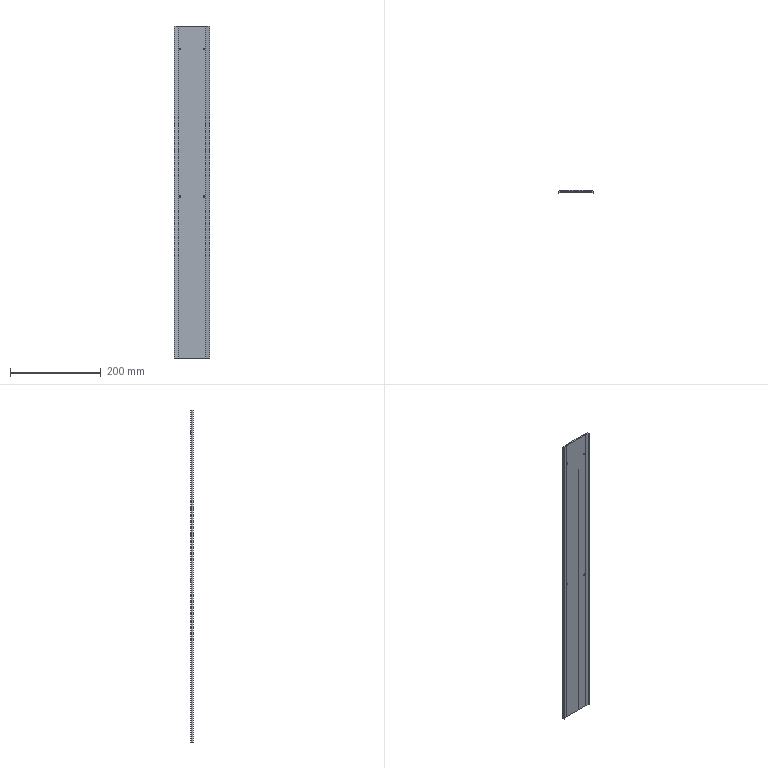Part | NX | 1 solid | 37 faces | box 79 x 6 x 732 mm | volume 149566 mm3 | plane 29 | cylinder 4 | cone 4 | commonest cylinder face diameters 3.4 x4
STEP:
#1=CARTESIAN_POINT('',(518.205,169.433,382.));
#2=VERTEX_POINT('',#1);
#3=CARTESIAN_POINT('',(518.205,165.108,382.));
#4=VERTEX_POINT('',#3);
#5=CARTESIAN_POINT('',(518.205,169.433,382.));
#6=DIRECTION('',(0.,-1.,0.));
#7=VECTOR('',#6,1.);
#8=LINE('',#5,#7);
#9=EDGE_CURVE('',#2,#4,#8,.T.);
#10=ORIENTED_EDGE('',*,*,#9,.F.);
#11=CARTESIAN_POINT('',(518.205,169.433,-350.));
#12=VERTEX_POINT('',#11);
#13=CARTESIAN_POINT('',(518.205,169.433,0.));
#14=DIRECTION('',(0.,0.,1.));
#15=VECTOR('',#14,1.);
#16=LINE('',#13,#15);
#17=EDGE_CURVE('',#12,#2,#16,.T.);
#18=ORIENTED_EDGE('',*,*,#17,.F.);
#19=CARTESIAN_POINT('',(518.205,165.108,-350.));
#20=VERTEX_POINT('',#19);
#21=CARTESIAN_POINT('',(518.205,0.,-350.));
#22=DIRECTION('',(0.,-1.,0.));
#23=VECTOR('',#22,1.);
#24=LINE('',#21,#23);
#25=EDGE_CURVE('',#12,#20,#24,.T.);
#26=ORIENTED_EDGE('',*,*,#25,.T.);
#27=CARTESIAN_POINT('',(518.205,165.108,0.));
#28=DIRECTION('',(0.,0.,1.));
#29=VECTOR('',#28,1.);
#30=LINE('',#27,#29);
#31=EDGE_CURVE('',#20,#4,#30,.T.);
#32=ORIENTED_EDGE('',*,*,#31,.T.);
#33=EDGE_LOOP('',(#10,#18,#26,#32));
#34=FACE_OUTER_BOUND('',#33,.T.);
#35=CARTESIAN_POINT('',(518.205,169.433,0.));
#36=DIRECTION('',(-1.,0.,0.));
#37=DIRECTION('',(0.,0.,-1.));
#38=AXIS2_PLACEMENT_3D('',#35,#36,#37);
#39=PLANE('',#38);
#40=ADVANCED_FACE('',(#34),#39,.T.);
#41=CARTESIAN_POINT('',(520.205,165.108,382.));
#42=VERTEX_POINT('',#41);
#43=CARTESIAN_POINT('',(518.205,165.108,382.));
#44=DIRECTION('',(1.,0.,0.));
#45=VECTOR('',#44,1.);
#46=LINE('',#43,#45);
#47=EDGE_CURVE('',#4,#42,#46,.T.);
#48=ORIENTED_EDGE('',*,*,#47,.F.);
#49=ORIENTED_EDGE('',*,*,#31,.F.);
#50=CARTESIAN_POINT('',(520.205,165.108,-350.));
#51=VERTEX_POINT('',#50);
#52=CARTESIAN_POINT('',(0.,165.108,-350.));
#53=DIRECTION('',(1.,0.,0.));
#54=VECTOR('',#53,1.);
#55=LINE('',#52,#54);
#56=EDGE_CURVE('',#20,#51,#55,.T.);
#57=ORIENTED_EDGE('',*,*,#56,.T.);
#58=CARTESIAN_POINT('',(520.205,165.108,0.));
#59=DIRECTION('',(0.,0.,1.));
#60=VECTOR('',#59,1.);
#61=LINE('',#58,#60);
#62=EDGE_CURVE('',#51,#42,#61,.T.);
#63=ORIENTED_EDGE('',*,*,#62,.T.);
#64=EDGE_LOOP('',(#48,#49,#57,#63));
#65=FACE_OUTER_BOUND('',#64,.T.);
#66=CARTESIAN_POINT('',(518.205,165.108,0.));
#67=DIRECTION('',(0.,-1.,0.));
#68=DIRECTION('',(0.,0.,1.));
#69=AXIS2_PLACEMENT_3D('',#66,#67,#68);
#70=PLANE('',#69);
#71=ADVANCED_FACE('',(#65),#70,.T.);
#72=CARTESIAN_POINT('',(520.205,167.247,382.));
#73=VERTEX_POINT('',#72);
#74=CARTESIAN_POINT('',(520.205,165.108,382.));
#75=DIRECTION('',(0.,1.,0.));
#76=VECTOR('',#75,1.);
#77=LINE('',#74,#76);
#78=EDGE_CURVE('',#42,#73,#77,.T.);
#79=ORIENTED_EDGE('',*,*,#78,.F.);
#80=ORIENTED_EDGE('',*,*,#62,.F.);
#81=CARTESIAN_POINT('',(520.205,167.247,-350.));
#82=VERTEX_POINT('',#81);
#83=CARTESIAN_POINT('',(520.205,0.,-350.));
#84=DIRECTION('',(0.,1.,0.));
#85=VECTOR('',#84,1.);
#86=LINE('',#83,#85);
#87=EDGE_CURVE('',#51,#82,#86,.T.);
#88=ORIENTED_EDGE('',*,*,#87,.T.);
#89=CARTESIAN_POINT('',(520.205,167.247,0.));
#90=DIRECTION('',(0.,0.,1.));
#91=VECTOR('',#90,1.);
#92=LINE('',#89,#91);
#93=EDGE_CURVE('',#82,#73,#92,.T.);
#94=ORIENTED_EDGE('',*,*,#93,.T.);
#95=EDGE_LOOP('',(#79,#80,#88,#94));
#96=FACE_OUTER_BOUND('',#95,.T.);
#97=CARTESIAN_POINT('',(520.205,165.108,0.));
#98=DIRECTION('',(1.,0.,0.));
#99=DIRECTION('',(0.,0.,1.));
#100=AXIS2_PLACEMENT_3D('',#97,#98,#99);
#101=PLANE('',#100);
#102=ADVANCED_FACE('',(#96),#101,.T.);
#103=CARTESIAN_POINT('',(527.924,168.608,382.));
#104=VERTEX_POINT('',#103);
#105=CARTESIAN_POINT('',(520.205,167.247,382.));
#106=DIRECTION('',(0.9848,0.1736,0.));
#107=VECTOR('',#106,1.);
#108=LINE('',#105,#107);
#109=EDGE_CURVE('',#73,#104,#108,.T.);
#110=ORIENTED_EDGE('',*,*,#109,.F.);
#111=ORIENTED_EDGE('',*,*,#93,.F.);
#112=CARTESIAN_POINT('',(527.924,168.608,-350.));
#113=VERTEX_POINT('',#112);
#114=CARTESIAN_POINT('',(-12.915,73.244,-350.));
#115=DIRECTION('',(0.9848,0.1736,0.));
#116=VECTOR('',#115,1.);
#117=LINE('',#114,#116);
#118=EDGE_CURVE('',#82,#113,#117,.T.);
#119=ORIENTED_EDGE('',*,*,#118,.T.);
#120=CARTESIAN_POINT('',(527.924,168.608,0.));
#121=DIRECTION('',(0.,0.,1.));
#122=VECTOR('',#121,1.);
#123=LINE('',#120,#122);
#124=EDGE_CURVE('',#113,#104,#123,.T.);
#125=ORIENTED_EDGE('',*,*,#124,.T.);
#126=EDGE_LOOP('',(#110,#111,#119,#125));
#127=FACE_OUTER_BOUND('',#126,.T.);
#128=CARTESIAN_POINT('',(520.205,167.247,0.));
#129=DIRECTION('',(0.1736,-0.9848,0.));
#130=DIRECTION('',(-0.9848,-0.1736,0.));
#131=AXIS2_PLACEMENT_3D('',#128,#129,#130);
#132=PLANE('',#131);
#133=ADVANCED_FACE('',(#127),#132,.T.);
#134=CARTESIAN_POINT('',(531.705,168.608,329.8));
#135=VERTEX_POINT('',#134);
#136=CARTESIAN_POINT('',(531.705,168.608,331.5));
#137=DIRECTION('',(0.,-1.,0.));
#138=DIRECTION('',(0.,0.,-1.));
#139=AXIS2_PLACEMENT_3D('',#136,#137,#138);
#140=CIRCLE('',#139,1.7);
#141=EDGE_CURVE('',#135,#135,#140,.T.);
#142=ORIENTED_EDGE('',*,*,#141,.F.);
#143=EDGE_LOOP('',(#142));
#144=FACE_BOUND('',#143,.T.);
#145=CARTESIAN_POINT('',(583.705,168.608,4.3));
#146=VERTEX_POINT('',#145);
#147=CARTESIAN_POINT('',(583.705,168.608,6.));
#148=DIRECTION('',(0.,-1.,0.));
#149=DIRECTION('',(0.,0.,-1.));
#150=AXIS2_PLACEMENT_3D('',#147,#148,#149);
#151=CIRCLE('',#150,1.7);
#152=EDGE_CURVE('',#146,#146,#151,.T.);
#153=ORIENTED_EDGE('',*,*,#152,.F.);
#154=EDGE_LOOP('',(#153));
#155=FACE_BOUND('',#154,.T.);
#156=CARTESIAN_POINT('',(583.705,168.608,329.8));
#157=VERTEX_POINT('',#156);
#158=CARTESIAN_POINT('',(583.705,168.608,331.5));
#159=DIRECTION('',(0.,-1.,0.));
#160=DIRECTION('',(0.,0.,-1.));
#161=AXIS2_PLACEMENT_3D('',#158,#159,#160);
#162=CIRCLE('',#161,1.7);
#163=EDGE_CURVE('',#157,#157,#162,.T.);
#164=ORIENTED_EDGE('',*,*,#163,.F.);
#165=EDGE_LOOP('',(#164));
#166=FACE_BOUND('',#165,.T.);
#167=CARTESIAN_POINT('',(531.705,168.608,4.3));
#168=VERTEX_POINT('',#167);
#169=CARTESIAN_POINT('',(531.705,168.608,6.));
#170=DIRECTION('',(0.,-1.,0.));
#171=DIRECTION('',(0.,0.,-1.));
#172=AXIS2_PLACEMENT_3D('',#169,#170,#171);
#173=CIRCLE('',#172,1.7);
#174=EDGE_CURVE('',#168,#168,#173,.T.);
#175=ORIENTED_EDGE('',*,*,#174,.F.);
#176=EDGE_LOOP('',(#175));
#177=FACE_BOUND('',#176,.T.);
#178=CARTESIAN_POINT('',(587.487,168.608,382.));
#179=VERTEX_POINT('',#178);
#180=CARTESIAN_POINT('',(527.924,168.608,382.));
#181=DIRECTION('',(1.,0.,0.));
#182=VECTOR('',#181,1.);
#183=LINE('',#180,#182);
#184=EDGE_CURVE('',#104,#179,#183,.T.);
#185=ORIENTED_EDGE('',*,*,#184,.F.);
#186=ORIENTED_EDGE('',*,*,#124,.F.);
#187=CARTESIAN_POINT('',(587.487,168.608,-350.));
#188=VERTEX_POINT('',#187);
#189=CARTESIAN_POINT('',(0.,168.608,-350.));
#190=DIRECTION('',(1.,0.,0.));
#191=VECTOR('',#190,1.);
#192=LINE('',#189,#191);
#193=EDGE_CURVE('',#113,#188,#192,.T.);
#194=ORIENTED_EDGE('',*,*,#193,.T.);
#195=CARTESIAN_POINT('',(587.487,168.608,0.));
#196=DIRECTION('',(0.,0.,1.));
#197=VECTOR('',#196,1.);
#198=LINE('',#195,#197);
#199=EDGE_CURVE('',#188,#179,#198,.T.);
#200=ORIENTED_EDGE('',*,*,#199,.T.);
#201=EDGE_LOOP('',(#185,#186,#194,#200));
#202=FACE_BOUND('',#201,.T.);
#203=CARTESIAN_POINT('',(527.924,168.608,0.));
#204=DIRECTION('',(0.,-1.,0.));
#205=DIRECTION('',(0.,0.,1.));
#206=AXIS2_PLACEMENT_3D('',#203,#204,#205);
#207=PLANE('',#206);
#208=ADVANCED_FACE('',(#144,#155,#166,#177,#202),#207,.T.);
#209=CARTESIAN_POINT('',(595.205,167.247,382.));
#210=VERTEX_POINT('',#209);
#211=CARTESIAN_POINT('',(587.487,168.608,382.));
#212=DIRECTION('',(0.9848,-0.1736,0.));
#213=VECTOR('',#212,1.);
#214=LINE('',#211,#213);
#215=EDGE_CURVE('',#179,#210,#214,.T.);
#216=ORIENTED_EDGE('',*,*,#215,.F.);
#217=ORIENTED_EDGE('',*,*,#199,.F.);
#218=CARTESIAN_POINT('',(595.205,167.247,-350.));
#219=VERTEX_POINT('',#218);
#220=CARTESIAN_POINT('',(46.549,263.99,-350.));
#221=DIRECTION('',(0.9848,-0.1736,0.));
#222=VECTOR('',#221,1.);
#223=LINE('',#220,#222);
#224=EDGE_CURVE('',#188,#219,#223,.T.);
#225=ORIENTED_EDGE('',*,*,#224,.T.);
#226=CARTESIAN_POINT('',(595.205,167.247,0.));
#227=DIRECTION('',(0.,0.,1.));
#228=VECTOR('',#227,1.);
#229=LINE('',#226,#228);
#230=EDGE_CURVE('',#219,#210,#229,.T.);
#231=ORIENTED_EDGE('',*,*,#230,.T.);
#232=EDGE_LOOP('',(#216,#217,#225,#231));
#233=FACE_OUTER_BOUND('',#232,.T.);
#234=CARTESIAN_POINT('',(587.487,168.608,0.));
#235=DIRECTION('',(-0.1736,-0.9848,0.));
#236=DIRECTION('',(-0.9848,0.1736,0.));
#237=AXIS2_PLACEMENT_3D('',#234,#235,#236);
#238=PLANE('',#237);
#239=ADVANCED_FACE('',(#233),#238,.T.);
#240=CARTESIAN_POINT('',(595.205,165.108,382.));
#241=VERTEX_POINT('',#240);
#242=CARTESIAN_POINT('',(595.205,167.247,382.));
#243=DIRECTION('',(0.,-1.,0.));
#244=VECTOR('',#243,1.);
#245=LINE('',#242,#244);
#246=EDGE_CURVE('',#210,#241,#245,.T.);
#247=ORIENTED_EDGE('',*,*,#246,.F.);
#248=ORIENTED_EDGE('',*,*,#230,.F.);
#249=CARTESIAN_POINT('',(595.205,165.108,-350.));
#250=VERTEX_POINT('',#249);
#251=CARTESIAN_POINT('',(595.205,0.,-350.));
#252=DIRECTION('',(0.,-1.,0.));
#253=VECTOR('',#252,1.);
#254=LINE('',#251,#253);
#255=EDGE_CURVE('',#219,#250,#254,.T.);
#256=ORIENTED_EDGE('',*,*,#255,.T.);
#257=CARTESIAN_POINT('',(595.205,165.108,0.));
#258=DIRECTION('',(0.,0.,1.));
#259=VECTOR('',#258,1.);
#260=LINE('',#257,#259);
#261=EDGE_CURVE('',#250,#241,#260,.T.);
#262=ORIENTED_EDGE('',*,*,#261,.T.);
#263=EDGE_LOOP('',(#247,#248,#256,#262));
#264=FACE_OUTER_BOUND('',#263,.T.);
#265=CARTESIAN_POINT('',(595.205,167.247,0.));
#266=DIRECTION('',(-1.,0.,0.));
#267=DIRECTION('',(0.,0.,-1.));
#268=AXIS2_PLACEMENT_3D('',#265,#266,#267);
#269=PLANE('',#268);
#270=ADVANCED_FACE('',(#264),#269,.T.);
#271=CARTESIAN_POINT('',(597.205,165.108,382.));
#272=VERTEX_POINT('',#271);
#273=CARTESIAN_POINT('',(595.205,165.108,382.));
#274=DIRECTION('',(1.,0.,0.));
#275=VECTOR('',#274,1.);
#276=LINE('',#273,#275);
#277=EDGE_CURVE('',#241,#272,#276,.T.);
#278=ORIENTED_EDGE('',*,*,#277,.F.);
#279=ORIENTED_EDGE('',*,*,#261,.F.);
#280=CARTESIAN_POINT('',(597.205,165.108,-350.));
#281=VERTEX_POINT('',#280);
#282=CARTESIAN_POINT('',(0.,165.108,-350.));
#283=DIRECTION('',(1.,0.,0.));
#284=VECTOR('',#283,1.);
#285=LINE('',#282,#284);
#286=EDGE_CURVE('',#250,#281,#285,.T.);
#287=ORIENTED_EDGE('',*,*,#286,.T.);
#288=CARTESIAN_POINT('',(597.205,165.108,0.));
#289=DIRECTION('',(0.,0.,1.));
#290=VECTOR('',#289,1.);
#291=LINE('',#288,#290);
#292=EDGE_CURVE('',#281,#272,#291,.T.);
#293=ORIENTED_EDGE('',*,*,#292,.T.);
#294=EDGE_LOOP('',(#278,#279,#287,#293));
#295=FACE_OUTER_BOUND('',#294,.T.);
#296=CARTESIAN_POINT('',(595.205,165.108,0.));
#297=DIRECTION('',(0.,-1.,0.));
#298=DIRECTION('',(0.,0.,1.));
#299=AXIS2_PLACEMENT_3D('',#296,#297,#298);
#300=PLANE('',#299);
#301=ADVANCED_FACE('',(#295),#300,.T.);
#302=CARTESIAN_POINT('',(597.205,169.433,382.));
#303=VERTEX_POINT('',#302);
#304=CARTESIAN_POINT('',(597.205,165.108,382.));
#305=DIRECTION('',(0.,1.,0.));
#306=VECTOR('',#305,1.);
#307=LINE('',#304,#306);
#308=EDGE_CURVE('',#272,#303,#307,.T.);
#309=ORIENTED_EDGE('',*,*,#308,.F.);
#310=ORIENTED_EDGE('',*,*,#292,.F.);
#311=CARTESIAN_POINT('',(597.205,169.433,-350.));
#312=VERTEX_POINT('',#311);
#313=CARTESIAN_POINT('',(597.205,0.,-350.));
#314=DIRECTION('',(0.,1.,0.));
#315=VECTOR('',#314,1.);
#316=LINE('',#313,#315);
#317=EDGE_CURVE('',#281,#312,#316,.T.);
#318=ORIENTED_EDGE('',*,*,#317,.T.);
#319=CARTESIAN_POINT('',(597.205,169.433,0.));
#320=DIRECTION('',(0.,0.,1.));
#321=VECTOR('',#320,1.);
#322=LINE('',#319,#321);
#323=EDGE_CURVE('',#312,#303,#322,.T.);
#324=ORIENTED_EDGE('',*,*,#323,.T.);
#325=EDGE_LOOP('',(#309,#310,#318,#324));
#326=FACE_OUTER_BOUND('',#325,.T.);
#327=CARTESIAN_POINT('',(597.205,165.108,0.));
#328=DIRECTION('',(1.,0.,0.));
#329=DIRECTION('',(0.,0.,1.));
#330=AXIS2_PLACEMENT_3D('',#327,#328,#329);
#331=PLANE('',#330);
#332=ADVANCED_FACE('',(#326),#331,.T.);
#333=CARTESIAN_POINT('',(587.705,171.108,382.));
#334=VERTEX_POINT('',#333);
#335=CARTESIAN_POINT('',(597.205,169.433,382.));
#336=DIRECTION('',(-0.9848,0.1736,0.));
#337=VECTOR('',#336,1.);
#338=LINE('',#335,#337);
#339=EDGE_CURVE('',#303,#334,#338,.T.);
#340=ORIENTED_EDGE('',*,*,#339,.F.);
#341=ORIENTED_EDGE('',*,*,#323,.F.);
#342=CARTESIAN_POINT('',(587.705,171.108,-350.));
#343=VERTEX_POINT('',#342);
#344=CARTESIAN_POINT('',(46.983,266.452,-350.));
#345=DIRECTION('',(-0.9848,0.1736,0.));
#346=VECTOR('',#345,1.);
#347=LINE('',#344,#346);
#348=EDGE_CURVE('',#312,#343,#347,.T.);
#349=ORIENTED_EDGE('',*,*,#348,.T.);
#350=CARTESIAN_POINT('',(587.705,171.108,0.));
#351=DIRECTION('',(0.,0.,1.));
#352=VECTOR('',#351,1.);
#353=LINE('',#350,#352);
#354=EDGE_CURVE('',#343,#334,#353,.T.);
#355=ORIENTED_EDGE('',*,*,#354,.T.);
#356=EDGE_LOOP('',(#340,#341,#349,#355));
#357=FACE_OUTER_BOUND('',#356,.T.);
#358=CARTESIAN_POINT('',(597.205,169.433,0.));
#359=DIRECTION('',(0.1736,0.9848,0.));
#360=DIRECTION('',(0.9848,-0.1736,0.));
#361=AXIS2_PLACEMENT_3D('',#358,#359,#360);
#362=PLANE('',#361);
#363=ADVANCED_FACE('',(#357),#362,.T.);
#364=CARTESIAN_POINT('',(583.705,171.108,9.3));
#365=VERTEX_POINT('',#364);
#366=CARTESIAN_POINT('',(583.705,171.108,6.));
#367=DIRECTION('',(0.,-1.,0.));
#368=DIRECTION('',(0.,0.,1.));
#369=AXIS2_PLACEMENT_3D('',#366,#367,#368);
#370=CIRCLE('',#369,3.3);
#371=EDGE_CURVE('',#365,#365,#370,.T.);
#372=ORIENTED_EDGE('',*,*,#371,.T.);
#373=EDGE_LOOP('',(#372));
#374=FACE_BOUND('',#373,.T.);
#375=CARTESIAN_POINT('',(583.705,171.108,334.8));
#376=VERTEX_POINT('',#375);
#377=CARTESIAN_POINT('',(583.705,171.108,331.5));
#378=DIRECTION('',(0.,-1.,0.));
#379=DIRECTION('',(0.,0.,1.));
#380=AXIS2_PLACEMENT_3D('',#377,#378,#379);
#381=CIRCLE('',#380,3.3);
#382=EDGE_CURVE('',#376,#376,#381,.T.);
#383=ORIENTED_EDGE('',*,*,#382,.T.);
#384=EDGE_LOOP('',(#383));
#385=FACE_BOUND('',#384,.T.);
#386=CARTESIAN_POINT('',(568.323,171.108,382.));
#387=VERTEX_POINT('',#386);
#388=CARTESIAN_POINT('',(587.705,171.108,382.));
#389=DIRECTION('',(-1.,0.,0.));
#390=VECTOR('',#389,1.);
#391=LINE('',#388,#390);
#392=EDGE_CURVE('',#334,#387,#391,.T.);
#393=ORIENTED_EDGE('',*,*,#392,.F.);
#394=ORIENTED_EDGE('',*,*,#354,.F.);
#395=CARTESIAN_POINT('',(568.323,171.108,-350.));
#396=VERTEX_POINT('',#395);
#397=CARTESIAN_POINT('',(0.,171.108,-350.));
#398=DIRECTION('',(-1.,0.,0.));
#399=VECTOR('',#398,1.);
#400=LINE('',#397,#399);
#401=EDGE_CURVE('',#343,#396,#400,.T.);
#402=ORIENTED_EDGE('',*,*,#401,.T.);
#403=CARTESIAN_POINT('',(568.323,171.108,0.));
#404=DIRECTION('',(0.,0.,1.));
#405=VECTOR('',#404,1.);
#406=LINE('',#403,#405);
#407=EDGE_CURVE('',#396,#387,#406,.T.);
#408=ORIENTED_EDGE('',*,*,#407,.T.);
#409=EDGE_LOOP('',(#393,#394,#402,#408));
#410=FACE_BOUND('',#409,.T.);
#411=CARTESIAN_POINT('',(587.705,171.108,0.));
#412=DIRECTION('',(0.,1.,0.));
#413=DIRECTION('',(0.,0.,-1.));
#414=AXIS2_PLACEMENT_3D('',#411,#412,#413);
#415=PLANE('',#414);
#416=ADVANCED_FACE('',(#374,#385,#410),#415,.T.);
#417=CARTESIAN_POINT('',(567.705,170.608,382.));
#418=VERTEX_POINT('',#417);
#419=CARTESIAN_POINT('',(568.323,171.108,382.));
#420=DIRECTION('',(-0.7774,-0.629,0.));
#421=VECTOR('',#420,1.);
#422=LINE('',#419,#421);
#423=EDGE_CURVE('',#387,#418,#422,.T.);
#424=ORIENTED_EDGE('',*,*,#423,.F.);
#425=ORIENTED_EDGE('',*,*,#407,.F.);
#426=CARTESIAN_POINT('',(567.705,170.608,-350.));
#427=VERTEX_POINT('',#426);
#428=CARTESIAN_POINT('',(141.154,-174.477,-350.));
#429=DIRECTION('',(-0.7774,-0.629,0.));
#430=VECTOR('',#429,1.);
#431=LINE('',#428,#430);
#432=EDGE_CURVE('',#396,#427,#431,.T.);
#433=ORIENTED_EDGE('',*,*,#432,.T.);
#434=CARTESIAN_POINT('',(567.705,170.608,0.));
#435=DIRECTION('',(0.,0.,1.));
#436=VECTOR('',#435,1.);
#437=LINE('',#434,#436);
#438=EDGE_CURVE('',#427,#418,#437,.T.);
#439=ORIENTED_EDGE('',*,*,#438,.T.);
#440=EDGE_LOOP('',(#424,#425,#433,#439));
#441=FACE_OUTER_BOUND('',#440,.T.);
#442=CARTESIAN_POINT('',(568.323,171.108,0.));
#443=DIRECTION('',(-0.629,0.7774,0.));
#444=DIRECTION('',(0.7774,0.629,0.));
#445=AXIS2_PLACEMENT_3D('',#442,#443,#444);
#446=PLANE('',#445);
#447=ADVANCED_FACE('',(#441),#446,.T.);
#448=CARTESIAN_POINT('',(567.087,171.108,382.));
#449=VERTEX_POINT('',#448);
#450=CARTESIAN_POINT('',(567.705,170.608,382.));
#451=DIRECTION('',(-0.7774,0.629,0.));
#452=VECTOR('',#451,1.);
#453=LINE('',#450,#452);
#454=EDGE_CURVE('',#418,#449,#453,.T.);
#455=ORIENTED_EDGE('',*,*,#454,.F.);
#456=ORIENTED_EDGE('',*,*,#438,.F.);
#457=CARTESIAN_POINT('',(567.087,171.108,-350.));
#458=VERTEX_POINT('',#457);
#459=CARTESIAN_POINT('',(308.001,380.712,-350.));
#460=DIRECTION('',(-0.7774,0.629,0.));
#461=VECTOR('',#460,1.);
#462=LINE('',#459,#461);
#463=EDGE_CURVE('',#427,#458,#462,.T.);
#464=ORIENTED_EDGE('',*,*,#463,.T.);
#465=CARTESIAN_POINT('',(567.087,171.108,0.));
#466=DIRECTION('',(0.,0.,1.));
#467=VECTOR('',#466,1.);
#468=LINE('',#465,#467);
#469=EDGE_CURVE('',#458,#449,#468,.T.);
#470=ORIENTED_EDGE('',*,*,#469,.T.);
#471=EDGE_LOOP('',(#455,#456,#464,#470));
#472=FACE_OUTER_BOUND('',#471,.T.);
#473=CARTESIAN_POINT('',(567.705,170.608,0.));
#474=DIRECTION('',(0.629,0.7774,0.));
#475=DIRECTION('',(0.7774,-0.629,0.));
#476=AXIS2_PLACEMENT_3D('',#473,#474,#475);
#477=PLANE('',#476);
#478=ADVANCED_FACE('',(#472),#477,.T.);
#479=CARTESIAN_POINT('',(563.323,171.108,382.));
#480=VERTEX_POINT('',#479);
#481=CARTESIAN_POINT('',(567.087,171.108,382.));
#482=DIRECTION('',(-1.,0.,0.));
#483=VECTOR('',#482,1.);
#484=LINE('',#481,#483);
#485=EDGE_CURVE('',#449,#480,#484,.T.);
#486=ORIENTED_EDGE('',*,*,#485,.F.);
#487=ORIENTED_EDGE('',*,*,#469,.F.);
#488=CARTESIAN_POINT('',(563.323,171.108,-350.));
#489=VERTEX_POINT('',#488);
#490=CARTESIAN_POINT('',(0.,171.108,-350.));
#491=DIRECTION('',(-1.,0.,0.));
#492=VECTOR('',#491,1.);
#493=LINE('',#490,#492);
#494=EDGE_CURVE('',#458,#489,#493,.T.);
#495=ORIENTED_EDGE('',*,*,#494,.T.);
#496=CARTESIAN_POINT('',(563.323,171.108,0.));
#497=DIRECTION('',(0.,0.,1.));
#498=VECTOR('',#497,1.);
#499=LINE('',#496,#498);
#500=EDGE_CURVE('',#489,#480,#499,.T.);
#501=ORIENTED_EDGE('',*,*,#500,.T.);
#502=EDGE_LOOP('',(#486,#487,#495,#501));
#503=FACE_OUTER_BOUND('',#502,.T.);
#504=CARTESIAN_POINT('',(567.087,171.108,0.));
#505=DIRECTION('',(0.,1.,0.));
#506=DIRECTION('',(0.,0.,-1.));
#507=AXIS2_PLACEMENT_3D('',#504,#505,#506);
#508=PLANE('',#507);
#509=ADVANCED_FACE('',(#503),#508,.T.);
#510=CARTESIAN_POINT('',(562.705,170.608,382.));
#511=VERTEX_POINT('',#510);
#512=CARTESIAN_POINT('',(563.323,171.108,382.));
#513=DIRECTION('',(-0.7774,-0.629,0.));
#514=VECTOR('',#513,1.);
#515=LINE('',#512,#514);
#516=EDGE_CURVE('',#480,#511,#515,.T.);
#517=ORIENTED_EDGE('',*,*,#516,.F.);
#518=ORIENTED_EDGE('',*,*,#500,.F.);
#519=CARTESIAN_POINT('',(562.705,170.608,-350.));
#520=VERTEX_POINT('',#519);
#521=CARTESIAN_POINT('',(139.176,-172.032,-350.));
#522=DIRECTION('',(-0.7774,-0.629,0.));
#523=VECTOR('',#522,1.);
#524=LINE('',#521,#523);
#525=EDGE_CURVE('',#489,#520,#524,.T.);
#526=ORIENTED_EDGE('',*,*,#525,.T.);
#527=CARTESIAN_POINT('',(562.705,170.608,0.));
#528=DIRECTION('',(0.,0.,1.));
#529=VECTOR('',#528,1.);
#530=LINE('',#527,#529);
#531=EDGE_CURVE('',#520,#511,#530,.T.);
#532=ORIENTED_EDGE('',*,*,#531,.T.);
#533=EDGE_LOOP('',(#517,#518,#526,#532));
#534=FACE_OUTER_BOUND('',#533,.T.);
#535=CARTESIAN_POINT('',(563.323,171.108,0.));
#536=DIRECTION('',(-0.629,0.7774,0.));
#537=DIRECTION('',(0.7774,0.629,0.));
#538=AXIS2_PLACEMENT_3D('',#535,#536,#537);
#539=PLANE('',#538);
#540=ADVANCED_FACE('',(#534),#539,.T.);
#541=CARTESIAN_POINT('',(562.087,171.108,382.));
#542=VERTEX_POINT('',#541);
#543=CARTESIAN_POINT('',(562.705,170.608,382.));
#544=DIRECTION('',(-0.7774,0.629,0.));
#545=VECTOR('',#544,1.);
#546=LINE('',#543,#545);
#547=EDGE_CURVE('',#511,#542,#546,.T.);
#548=ORIENTED_EDGE('',*,*,#547,.F.);
#549=ORIENTED_EDGE('',*,*,#531,.F.);
#550=CARTESIAN_POINT('',(562.087,171.108,-350.));
#551=VERTEX_POINT('',#550);
#552=CARTESIAN_POINT('',(306.023,378.267,-350.));
#553=DIRECTION('',(-0.7774,0.629,0.));
#554=VECTOR('',#553,1.);
#555=LINE('',#552,#554);
#556=EDGE_CURVE('',#520,#551,#555,.T.);
#557=ORIENTED_EDGE('',*,*,#556,.T.);
#558=CARTESIAN_POINT('',(562.087,171.108,0.));
#559=DIRECTION('',(0.,0.,1.));
#560=VECTOR('',#559,1.);
#561=LINE('',#558,#560);
#562=EDGE_CURVE('',#551,#542,#561,.T.);
#563=ORIENTED_EDGE('',*,*,#562,.T.);
#564=EDGE_LOOP('',(#548,#549,#557,#563));
#565=FACE_OUTER_BOUND('',#564,.T.);
#566=CARTESIAN_POINT('',(562.705,170.608,0.));
#567=DIRECTION('',(0.629,0.7774,0.));
#568=DIRECTION('',(0.7774,-0.629,0.));
#569=AXIS2_PLACEMENT_3D('',#566,#567,#568);
#570=PLANE('',#569);
#571=ADVANCED_FACE('',(#565),#570,.T.);
#572=CARTESIAN_POINT('',(558.323,171.108,382.));
#573=VERTEX_POINT('',#572);
#574=CARTESIAN_POINT('',(562.087,171.108,382.));
#575=DIRECTION('',(-1.,0.,0.));
#576=VECTOR('',#575,1.);
#577=LINE('',#574,#576);
#578=EDGE_CURVE('',#542,#573,#577,.T.);
#579=ORIENTED_EDGE('',*,*,#578,.F.);
#580=ORIENTED_EDGE('',*,*,#562,.F.);
#581=CARTESIAN_POINT('',(558.323,171.108,-350.));
#582=VERTEX_POINT('',#581);
#583=CARTESIAN_POINT('',(0.,171.108,-350.));
#584=DIRECTION('',(-1.,0.,0.));
#585=VECTOR('',#584,1.);
#586=LINE('',#583,#585);
#587=EDGE_CURVE('',#551,#582,#586,.T.);
#588=ORIENTED_EDGE('',*,*,#587,.T.);
#589=CARTESIAN_POINT('',(558.323,171.108,0.));
#590=DIRECTION('',(0.,0.,1.));
#591=VECTOR('',#590,1.);
#592=LINE('',#589,#591);
#593=EDGE_CURVE('',#582,#573,#592,.T.);
#594=ORIENTED_EDGE('',*,*,#593,.T.);
#595=EDGE_LOOP('',(#579,#580,#588,#594));
#596=FACE_OUTER_BOUND('',#595,.T.);
#597=CARTESIAN_POINT('',(562.087,171.108,0.));
#598=DIRECTION('',(0.,1.,0.));
#599=DIRECTION('',(0.,0.,-1.));
#600=AXIS2_PLACEMENT_3D('',#597,#598,#599);
#601=PLANE('',#600);
#602=ADVANCED_FACE('',(#596),#601,.T.);
#603=CARTESIAN_POINT('',(557.705,170.608,382.));
#604=VERTEX_POINT('',#603);
#605=CARTESIAN_POINT('',(558.323,171.108,382.));
#606=DIRECTION('',(-0.7774,-0.629,0.));
#607=VECTOR('',#606,1.);
#608=LINE('',#605,#607);
#609=EDGE_CURVE('',#573,#604,#608,.T.);
#610=ORIENTED_EDGE('',*,*,#609,.F.);
#611=ORIENTED_EDGE('',*,*,#593,.F.);
#612=CARTESIAN_POINT('',(557.705,170.608,-350.));
#613=VERTEX_POINT('',#612);
#614=CARTESIAN_POINT('',(137.199,-169.588,-350.));
#615=DIRECTION('',(-0.7774,-0.629,0.));
#616=VECTOR('',#615,1.);
#617=LINE('',#614,#616);
#618=EDGE_CURVE('',#582,#613,#617,.T.);
#619=ORIENTED_EDGE('',*,*,#618,.T.);
#620=CARTESIAN_POINT('',(557.705,170.608,0.));
#621=DIRECTION('',(0.,0.,1.));
#622=VECTOR('',#621,1.);
#623=LINE('',#620,#622);
#624=EDGE_CURVE('',#613,#604,#623,.T.);
#625=ORIENTED_EDGE('',*,*,#624,.T.);
#626=EDGE_LOOP('',(#610,#611,#619,#625));
#627=FACE_OUTER_BOUND('',#626,.T.);
#628=CARTESIAN_POINT('',(558.323,171.108,0.));
#629=DIRECTION('',(-0.629,0.7774,0.));
#630=DIRECTION('',(0.7774,0.629,0.));
#631=AXIS2_PLACEMENT_3D('',#628,#629,#630);
#632=PLANE('',#631);
#633=ADVANCED_FACE('',(#627),#632,.T.);
#634=CARTESIAN_POINT('',(557.087,171.108,382.));
#635=VERTEX_POINT('',#634);
#636=CARTESIAN_POINT('',(557.705,170.608,382.));
#637=DIRECTION('',(-0.7774,0.629,0.));
#638=VECTOR('',#637,1.);
#639=LINE('',#636,#638);
#640=EDGE_CURVE('',#604,#635,#639,.T.);
#641=ORIENTED_EDGE('',*,*,#640,.F.);
#642=ORIENTED_EDGE('',*,*,#624,.F.);
#643=CARTESIAN_POINT('',(557.087,171.108,-350.));
#644=VERTEX_POINT('',#643);
#645=CARTESIAN_POINT('',(304.045,375.822,-350.));
#646=DIRECTION('',(-0.7774,0.629,0.));
#647=VECTOR('',#646,1.);
#648=LINE('',#645,#647);
#649=EDGE_CURVE('',#613,#644,#648,.T.);
#650=ORIENTED_EDGE('',*,*,#649,.T.);
#651=CARTESIAN_POINT('',(557.087,171.108,0.));
#652=DIRECTION('',(0.,0.,1.));
#653=VECTOR('',#652,1.);
#654=LINE('',#651,#653);
#655=EDGE_CURVE('',#644,#635,#654,.T.);
#656=ORIENTED_EDGE('',*,*,#655,.T.);
#657=EDGE_LOOP('',(#641,#642,#650,#656));
#658=FACE_OUTER_BOUND('',#657,.T.);
#659=CARTESIAN_POINT('',(557.705,170.608,0.));
#660=DIRECTION('',(0.629,0.7774,0.));
#661=DIRECTION('',(0.7774,-0.629,0.));
#662=AXIS2_PLACEMENT_3D('',#659,#660,#661);
#663=PLANE('',#662);
#664=ADVANCED_FACE('',(#658),#663,.T.);
#665=CARTESIAN_POINT('',(553.323,171.108,382.));
#666=VERTEX_POINT('',#665);
#667=CARTESIAN_POINT('',(557.087,171.108,382.));
#668=DIRECTION('',(-1.,0.,0.));
#669=VECTOR('',#668,1.);
#670=LINE('',#667,#669);
#671=EDGE_CURVE('',#635,#666,#670,.T.);
#672=ORIENTED_EDGE('',*,*,#671,.F.);
#673=ORIENTED_EDGE('',*,*,#655,.F.);
#674=CARTESIAN_POINT('',(553.323,171.108,-350.));
#675=VERTEX_POINT('',#674);
#676=CARTESIAN_POINT('',(0.,171.108,-350.));
#677=DIRECTION('',(-1.,0.,0.));
#678=VECTOR('',#677,1.);
#679=LINE('',#676,#678);
#680=EDGE_CURVE('',#644,#675,#679,.T.);
#681=ORIENTED_EDGE('',*,*,#680,.T.);
#682=CARTESIAN_POINT('',(553.323,171.108,0.));
#683=DIRECTION('',(0.,0.,1.));
#684=VECTOR('',#683,1.);
#685=LINE('',#682,#684);
#686=EDGE_CURVE('',#675,#666,#685,.T.);
#687=ORIENTED_EDGE('',*,*,#686,.T.);
#688=EDGE_LOOP('',(#672,#673,#681,#687));
#689=FACE_OUTER_BOUND('',#688,.T.);
#690=CARTESIAN_POINT('',(557.087,171.108,0.));
#691=DIRECTION('',(0.,1.,0.));
#692=DIRECTION('',(0.,0.,-1.));
#693=AXIS2_PLACEMENT_3D('',#690,#691,#692);
#694=PLANE('',#693);
#695=ADVANCED_FACE('',(#689),#694,.T.);
#696=CARTESIAN_POINT('',(552.705,170.608,382.));
#697=VERTEX_POINT('',#696);
#698=CARTESIAN_POINT('',(553.323,171.108,382.));
#699=DIRECTION('',(-0.7774,-0.629,0.));
#700=VECTOR('',#699,1.);
#701=LINE('',#698,#700);
#702=EDGE_CURVE('',#666,#697,#701,.T.);
#703=ORIENTED_EDGE('',*,*,#702,.F.);
#704=ORIENTED_EDGE('',*,*,#686,.F.);
#705=CARTESIAN_POINT('',(552.705,170.608,-350.));
#706=VERTEX_POINT('',#705);
#707=CARTESIAN_POINT('',(135.221,-167.143,-350.));
#708=DIRECTION('',(-0.7774,-0.629,0.));
#709=VECTOR('',#708,1.);
#710=LINE('',#707,#709);
#711=EDGE_CURVE('',#675,#706,#710,.T.);
#712=ORIENTED_EDGE('',*,*,#711,.T.);
#713=CARTESIAN_POINT('',(552.705,170.608,0.));
#714=DIRECTION('',(0.,0.,1.));
#715=VECTOR('',#714,1.);
#716=LINE('',#713,#715);
#717=EDGE_CURVE('',#706,#697,#716,.T.);
#718=ORIENTED_EDGE('',*,*,#717,.T.);
#719=EDGE_LOOP('',(#703,#704,#712,#718));
#720=FACE_OUTER_BOUND('',#719,.T.);
#721=CARTESIAN_POINT('',(553.323,171.108,0.));
#722=DIRECTION('',(-0.629,0.7774,0.));
#723=DIRECTION('',(0.7774,0.629,0.));
#724=AXIS2_PLACEMENT_3D('',#721,#722,#723);
#725=PLANE('',#724);
#726=ADVANCED_FACE('',(#720),#725,.T.);
#727=CARTESIAN_POINT('',(552.087,171.108,382.));
#728=VERTEX_POINT('',#727);
#729=CARTESIAN_POINT('',(552.705,170.608,382.));
#730=DIRECTION('',(-0.7774,0.629,0.));
#731=VECTOR('',#730,1.);
#732=LINE('',#729,#731);
#733=EDGE_CURVE('',#697,#728,#732,.T.);
#734=ORIENTED_EDGE('',*,*,#733,.F.);
#735=ORIENTED_EDGE('',*,*,#717,.F.);
#736=CARTESIAN_POINT('',(552.087,171.108,-350.));
#737=VERTEX_POINT('',#736);
#738=CARTESIAN_POINT('',(302.067,373.378,-350.));
#739=DIRECTION('',(-0.7774,0.629,0.));
#740=VECTOR('',#739,1.);
#741=LINE('',#738,#740);
#742=EDGE_CURVE('',#706,#737,#741,.T.);
#743=ORIENTED_EDGE('',*,*,#742,.T.);
#744=CARTESIAN_POINT('',(552.087,171.108,0.));
#745=DIRECTION('',(0.,0.,1.));
#746=VECTOR('',#745,1.);
#747=LINE('',#744,#746);
#748=EDGE_CURVE('',#737,#728,#747,.T.);
#749=ORIENTED_EDGE('',*,*,#748,.T.);
#750=EDGE_LOOP('',(#734,#735,#743,#749));
#751=FACE_OUTER_BOUND('',#750,.T.);
#752=CARTESIAN_POINT('',(552.705,170.608,0.));
#753=DIRECTION('',(0.629,0.7774,0.));
#754=DIRECTION('',(0.7774,-0.629,0.));
#755=AXIS2_PLACEMENT_3D('',#752,#753,#754);
#756=PLANE('',#755);
#757=ADVANCED_FACE('',(#751),#756,.T.);
#758=CARTESIAN_POINT('',(548.323,171.108,382.));
#759=VERTEX_POINT('',#758);
#760=CARTESIAN_POINT('',(552.087,171.108,382.));
#761=DIRECTION('',(-1.,0.,0.));
#762=VECTOR('',#761,1.);
#763=LINE('',#760,#762);
#764=EDGE_CURVE('',#728,#759,#763,.T.);
#765=ORIENTED_EDGE('',*,*,#764,.F.);
#766=ORIENTED_EDGE('',*,*,#748,.F.);
#767=CARTESIAN_POINT('',(548.323,171.108,-350.));
#768=VERTEX_POINT('',#767);
#769=CARTESIAN_POINT('',(0.,171.108,-350.));
#770=DIRECTION('',(-1.,0.,0.));
#771=VECTOR('',#770,1.);
#772=LINE('',#769,#771);
#773=EDGE_CURVE('',#737,#768,#772,.T.);
#774=ORIENTED_EDGE('',*,*,#773,.T.);
#775=CARTESIAN_POINT('',(548.323,171.108,0.));
#776=DIRECTION('',(0.,0.,1.));
#777=VECTOR('',#776,1.);
#778=LINE('',#775,#777);
#779=EDGE_CURVE('',#768,#759,#778,.T.);
#780=ORIENTED_EDGE('',*,*,#779,.T.);
#781=EDGE_LOOP('',(#765,#766,#774,#780));
#782=FACE_OUTER_BOUND('',#781,.T.);
#783=CARTESIAN_POINT('',(552.087,171.108,0.));
#784=DIRECTION('',(0.,1.,0.));
#785=DIRECTION('',(0.,0.,-1.));
#786=AXIS2_PLACEMENT_3D('',#783,#784,#785);
#787=PLANE('',#786);
#788=ADVANCED_FACE('',(#782),#787,.T.);
#789=CARTESIAN_POINT('',(547.705,170.608,382.));
#790=VERTEX_POINT('',#789);
#791=CARTESIAN_POINT('',(548.323,171.108,382.));
#792=DIRECTION('',(-0.7774,-0.629,0.));
#793=VECTOR('',#792,1.);
#794=LINE('',#791,#793);
#795=EDGE_CURVE('',#759,#790,#794,.T.);
#796=ORIENTED_EDGE('',*,*,#795,.F.);
#797=ORIENTED_EDGE('',*,*,#779,.F.);
#798=CARTESIAN_POINT('',(547.705,170.608,-350.));
#799=VERTEX_POINT('',#798);
#800=CARTESIAN_POINT('',(133.243,-164.698,-350.));
#801=DIRECTION('',(-0.7774,-0.629,0.));
#802=VECTOR('',#801,1.);
#803=LINE('',#800,#802);
#804=EDGE_CURVE('',#768,#799,#803,.T.);
#805=ORIENTED_EDGE('',*,*,#804,.T.);
#806=CARTESIAN_POINT('',(547.705,170.608,0.));
#807=DIRECTION('',(0.,0.,1.));
#808=VECTOR('',#807,1.);
#809=LINE('',#806,#808);
#810=EDGE_CURVE('',#799,#790,#809,.T.);
#811=ORIENTED_EDGE('',*,*,#810,.T.);
#812=EDGE_LOOP('',(#796,#797,#805,#811));
#813=FACE_OUTER_BOUND('',#812,.T.);
#814=CARTESIAN_POINT('',(548.323,171.108,0.));
#815=DIRECTION('',(-0.629,0.7774,0.));
#816=DIRECTION('',(0.7774,0.629,0.));
#817=AXIS2_PLACEMENT_3D('',#814,#815,#816);
#818=PLANE('',#817);
#819=ADVANCED_FACE('',(#813),#818,.T.);
#820=CARTESIAN_POINT('',(547.087,171.108,382.));
#821=VERTEX_POINT('',#820);
#822=CARTESIAN_POINT('',(547.705,170.608,382.));
#823=DIRECTION('',(-0.7774,0.629,0.));
#824=VECTOR('',#823,1.);
#825=LINE('',#822,#824);
#826=EDGE_CURVE('',#790,#821,#825,.T.);
#827=ORIENTED_EDGE('',*,*,#826,.F.);
#828=ORIENTED_EDGE('',*,*,#810,.F.);
#829=CARTESIAN_POINT('',(547.087,171.108,-350.));
#830=VERTEX_POINT('',#829);
#831=CARTESIAN_POINT('',(300.089,370.933,-350.));
#832=DIRECTION('',(-0.7774,0.629,0.));
#833=VECTOR('',#832,1.);
#834=LINE('',#831,#833);
#835=EDGE_CURVE('',#799,#830,#834,.T.);
#836=ORIENTED_EDGE('',*,*,#835,.T.);
#837=CARTESIAN_POINT('',(547.087,171.108,0.));
#838=DIRECTION('',(0.,0.,1.));
#839=VECTOR('',#838,1.);
#840=LINE('',#837,#839);
#841=EDGE_CURVE('',#830,#821,#840,.T.);
#842=ORIENTED_EDGE('',*,*,#841,.T.);
#843=EDGE_LOOP('',(#827,#828,#836,#842));
#844=FACE_OUTER_BOUND('',#843,.T.);
#845=CARTESIAN_POINT('',(547.705,170.608,0.));
#846=DIRECTION('',(0.629,0.7774,0.));
#847=DIRECTION('',(0.7774,-0.629,0.));
#848=AXIS2_PLACEMENT_3D('',#845,#846,#847);
#849=PLANE('',#848);
#850=ADVANCED_FACE('',(#844),#849,.T.);
#851=CARTESIAN_POINT('',(531.705,171.108,9.3));
#852=VERTEX_POINT('',#851);
#853=CARTESIAN_POINT('',(531.705,171.108,6.));
#854=DIRECTION('',(0.,-1.,0.));
#855=DIRECTION('',(0.,0.,1.));
#856=AXIS2_PLACEMENT_3D('',#853,#854,#855);
#857=CIRCLE('',#856,3.3);
#858=EDGE_CURVE('',#852,#852,#857,.T.);
#859=ORIENTED_EDGE('',*,*,#858,.T.);
#860=EDGE_LOOP('',(#859));
#861=FACE_BOUND('',#860,.T.);
#862=CARTESIAN_POINT('',(531.705,171.108,334.8));
#863=VERTEX_POINT('',#862);
#864=CARTESIAN_POINT('',(531.705,171.108,331.5));
#865=DIRECTION('',(0.,-1.,0.));
#866=DIRECTION('',(0.,0.,1.));
#867=AXIS2_PLACEMENT_3D('',#864,#865,#866);
#868=CIRCLE('',#867,3.3);
#869=EDGE_CURVE('',#863,#863,#868,.T.);
#870=ORIENTED_EDGE('',*,*,#869,.T.);
#871=EDGE_LOOP('',(#870));
#872=FACE_BOUND('',#871,.T.);
#873=CARTESIAN_POINT('',(527.705,171.108,382.));
#874=VERTEX_POINT('',#873);
#875=CARTESIAN_POINT('',(547.087,171.108,382.));
#876=DIRECTION('',(-1.,0.,0.));
#877=VECTOR('',#876,1.);
#878=LINE('',#875,#877);
#879=EDGE_CURVE('',#821,#874,#878,.T.);
#880=ORIENTED_EDGE('',*,*,#879,.F.);
#881=ORIENTED_EDGE('',*,*,#841,.F.);
#882=CARTESIAN_POINT('',(527.705,171.108,-350.));
#883=VERTEX_POINT('',#882);
#884=CARTESIAN_POINT('',(0.,171.108,-350.));
#885=DIRECTION('',(-1.,0.,0.));
#886=VECTOR('',#885,1.);
#887=LINE('',#884,#886);
#888=EDGE_CURVE('',#830,#883,#887,.T.);
#889=ORIENTED_EDGE('',*,*,#888,.T.);
#890=CARTESIAN_POINT('',(527.705,171.108,0.));
#891=DIRECTION('',(0.,0.,1.));
#892=VECTOR('',#891,1.);
#893=LINE('',#890,#892);
#894=EDGE_CURVE('',#883,#874,#893,.T.);
#895=ORIENTED_EDGE('',*,*,#894,.T.);
#896=EDGE_LOOP('',(#880,#881,#889,#895));
#897=FACE_BOUND('',#896,.T.);
#898=CARTESIAN_POINT('',(547.087,171.108,0.));
#899=DIRECTION('',(0.,1.,0.));
#900=DIRECTION('',(0.,0.,-1.));
#901=AXIS2_PLACEMENT_3D('',#898,#899,#900);
#902=PLANE('',#901);
#903=ADVANCED_FACE('',(#861,#872,#897),#902,.T.);
#904=CARTESIAN_POINT('',(527.705,171.108,382.));
#905=DIRECTION('',(-0.9848,-0.1736,0.));
#906=VECTOR('',#905,1.);
#907=LINE('',#904,#906);
#908=EDGE_CURVE('',#874,#2,#907,.T.);
#909=ORIENTED_EDGE('',*,*,#908,.F.);
#910=ORIENTED_EDGE('',*,*,#894,.F.);
#911=CARTESIAN_POINT('',(-13.349,75.706,-350.));
#912=DIRECTION('',(-0.9848,-0.1736,0.));
#913=VECTOR('',#912,1.);
#914=LINE('',#911,#913);
#915=EDGE_CURVE('',#883,#12,#914,.T.);
#916=ORIENTED_EDGE('',*,*,#915,.T.);
#917=ORIENTED_EDGE('',*,*,#17,.T.);
#918=EDGE_LOOP('',(#909,#910,#916,#917));
#919=FACE_OUTER_BOUND('',#918,.T.);
#920=CARTESIAN_POINT('',(527.705,171.108,0.));
#921=DIRECTION('',(-0.1736,0.9848,0.));
#922=DIRECTION('',(0.9848,0.1736,0.));
#923=AXIS2_PLACEMENT_3D('',#920,#921,#922);
#924=PLANE('',#923);
#925=ADVANCED_FACE('',(#919),#924,.T.);
#926=ORIENTED_EDGE('',*,*,#25,.F.);
#927=ORIENTED_EDGE('',*,*,#915,.F.);
#928=ORIENTED_EDGE('',*,*,#888,.F.);
#929=ORIENTED_EDGE('',*,*,#835,.F.);
#930=ORIENTED_EDGE('',*,*,#804,.F.);
#931=ORIENTED_EDGE('',*,*,#773,.F.);
#932=ORIENTED_EDGE('',*,*,#742,.F.);
#933=ORIENTED_EDGE('',*,*,#711,.F.);
#934=ORIENTED_EDGE('',*,*,#680,.F.);
#935=ORIENTED_EDGE('',*,*,#649,.F.);
#936=ORIENTED_EDGE('',*,*,#618,.F.);
#937=ORIENTED_EDGE('',*,*,#587,.F.);
#938=ORIENTED_EDGE('',*,*,#556,.F.);
#939=ORIENTED_EDGE('',*,*,#525,.F.);
#940=ORIENTED_EDGE('',*,*,#494,.F.);
#941=ORIENTED_EDGE('',*,*,#463,.F.);
#942=ORIENTED_EDGE('',*,*,#432,.F.);
#943=ORIENTED_EDGE('',*,*,#401,.F.);
#944=ORIENTED_EDGE('',*,*,#348,.F.);
#945=ORIENTED_EDGE('',*,*,#317,.F.);
#946=ORIENTED_EDGE('',*,*,#286,.F.);
#947=ORIENTED_EDGE('',*,*,#255,.F.);
#948=ORIENTED_EDGE('',*,*,#224,.F.);
#949=ORIENTED_EDGE('',*,*,#193,.F.);
#950=ORIENTED_EDGE('',*,*,#118,.F.);
#951=ORIENTED_EDGE('',*,*,#87,.F.);
#952=ORIENTED_EDGE('',*,*,#56,.F.);
#953=EDGE_LOOP('',(#926,#927,#928,#929,#930,#931,#932,#933,#934,#935,#936,#937,#938,#939,#940,#941,#942,#943,#944,#945,#946,#947,#948,#949,#950,#951,#952));
#954=FACE_OUTER_BOUND('',#953,.T.);
#955=CARTESIAN_POINT('',(0.,0.,-350.));
#956=DIRECTION('',(0.,0.,1.));
#957=DIRECTION('',(-1.,0.,0.));
#958=AXIS2_PLACEMENT_3D('',#955,#956,#957);
#959=PLANE('',#958);
#960=ADVANCED_FACE('',(#954),#959,.F.);
#961=ORIENTED_EDGE('',*,*,#9,.T.);
#962=ORIENTED_EDGE('',*,*,#47,.T.);
#963=ORIENTED_EDGE('',*,*,#78,.T.);
#964=ORIENTED_EDGE('',*,*,#109,.T.);
#965=ORIENTED_EDGE('',*,*,#184,.T.);
#966=ORIENTED_EDGE('',*,*,#215,.T.);
#967=ORIENTED_EDGE('',*,*,#246,.T.);
#968=ORIENTED_EDGE('',*,*,#277,.T.);
#969=ORIENTED_EDGE('',*,*,#308,.T.);
#970=ORIENTED_EDGE('',*,*,#339,.T.);
#971=ORIENTED_EDGE('',*,*,#392,.T.);
#972=ORIENTED_EDGE('',*,*,#423,.T.);
#973=ORIENTED_EDGE('',*,*,#454,.T.);
#974=ORIENTED_EDGE('',*,*,#485,.T.);
#975=ORIENTED_EDGE('',*,*,#516,.T.);
#976=ORIENTED_EDGE('',*,*,#547,.T.);
#977=ORIENTED_EDGE('',*,*,#578,.T.);
#978=ORIENTED_EDGE('',*,*,#609,.T.);
#979=ORIENTED_EDGE('',*,*,#640,.T.);
#980=ORIENTED_EDGE('',*,*,#671,.T.);
#981=ORIENTED_EDGE('',*,*,#702,.T.);
#982=ORIENTED_EDGE('',*,*,#733,.T.);
#983=ORIENTED_EDGE('',*,*,#764,.T.);
#984=ORIENTED_EDGE('',*,*,#795,.T.);
#985=ORIENTED_EDGE('',*,*,#826,.T.);
#986=ORIENTED_EDGE('',*,*,#879,.T.);
#987=ORIENTED_EDGE('',*,*,#908,.T.);
#988=EDGE_LOOP('',(#961,#962,#963,#964,#965,#966,#967,#968,#969,#970,#971,#972,#973,#974,#975,#976,#977,#978,#979,#980,#981,#982,#983,#984,#985,#986,#987));
#989=FACE_OUTER_BOUND('',#988,.T.);
#990=CARTESIAN_POINT('',(0.,0.,382.));
#991=DIRECTION('',(0.,0.,1.));
#992=DIRECTION('',(-1.,0.,0.));
#993=AXIS2_PLACEMENT_3D('',#990,#991,#992);
#994=PLANE('',#993);
#995=ADVANCED_FACE('',(#989),#994,.T.);
#996=CARTESIAN_POINT('',(531.705,169.508,7.7));
#997=VERTEX_POINT('',#996);
#998=CARTESIAN_POINT('',(531.705,169.508,6.));
#999=DIRECTION('',(0.,1.,0.));
#1000=DIRECTION('',(0.,0.,1.));
#1001=AXIS2_PLACEMENT_3D('',#998,#999,#1000);
#1002=CIRCLE('',#1001,1.7);
#1003=EDGE_CURVE('',#997,#997,#1002,.T.);
#1004=ORIENTED_EDGE('',*,*,#1003,.T.);
#1005=EDGE_LOOP('',(#1004));
#1006=FACE_BOUND('',#1005,.T.);
#1007=ORIENTED_EDGE('',*,*,#174,.T.);
#1008=EDGE_LOOP('',(#1007));
#1009=FACE_BOUND('',#1008,.T.);
#1010=CARTESIAN_POINT('',(531.705,221.108,6.));
#1011=DIRECTION('',(0.,-1.,0.));
#1012=DIRECTION('',(0.,0.,1.));
#1013=AXIS2_PLACEMENT_3D('',#1010,#1011,#1012);
#1014=CYLINDRICAL_SURFACE('',#1013,1.7);
#1015=ADVANCED_FACE('',(#1006,#1009),#1014,.F.);
#1016=CARTESIAN_POINT('',(531.705,169.508,333.2));
#1017=VERTEX_POINT('',#1016);
#1018=CARTESIAN_POINT('',(531.705,169.508,331.5));
#1019=DIRECTION('',(0.,1.,0.));
#1020=DIRECTION('',(0.,0.,1.));
#1021=AXIS2_PLACEMENT_3D('',#1018,#1019,#1020);
#1022=CIRCLE('',#1021,1.7);
#1023=EDGE_CURVE('',#1017,#1017,#1022,.T.);
#1024=ORIENTED_EDGE('',*,*,#1023,.T.);
#1025=EDGE_LOOP('',(#1024));
#1026=FACE_BOUND('',#1025,.T.);
#1027=ORIENTED_EDGE('',*,*,#141,.T.);
#1028=EDGE_LOOP('',(#1027));
#1029=FACE_BOUND('',#1028,.T.);
#1030=CARTESIAN_POINT('',(531.705,221.108,331.5));
#1031=DIRECTION('',(0.,-1.,0.));
#1032=DIRECTION('',(0.,0.,1.));
#1033=AXIS2_PLACEMENT_3D('',#1030,#1031,#1032);
#1034=CYLINDRICAL_SURFACE('',#1033,1.7);
#1035=ADVANCED_FACE('',(#1026,#1029),#1034,.F.);
#1036=CARTESIAN_POINT('',(583.705,169.508,333.2));
#1037=VERTEX_POINT('',#1036);
#1038=CARTESIAN_POINT('',(583.705,169.508,331.5));
#1039=DIRECTION('',(0.,1.,0.));
#1040=DIRECTION('',(0.,0.,1.));
#1041=AXIS2_PLACEMENT_3D('',#1038,#1039,#1040);
#1042=CIRCLE('',#1041,1.7);
#1043=EDGE_CURVE('',#1037,#1037,#1042,.T.);
#1044=ORIENTED_EDGE('',*,*,#1043,.T.);
#1045=EDGE_LOOP('',(#1044));
#1046=FACE_BOUND('',#1045,.T.);
#1047=ORIENTED_EDGE('',*,*,#163,.T.);
#1048=EDGE_LOOP('',(#1047));
#1049=FACE_BOUND('',#1048,.T.);
#1050=CARTESIAN_POINT('',(583.705,221.108,331.5));
#1051=DIRECTION('',(0.,-1.,0.));
#1052=DIRECTION('',(0.,0.,1.));
#1053=AXIS2_PLACEMENT_3D('',#1050,#1051,#1052);
#1054=CYLINDRICAL_SURFACE('',#1053,1.7);
#1055=ADVANCED_FACE('',(#1046,#1049),#1054,.F.);
#1056=CARTESIAN_POINT('',(583.705,169.508,7.7));
#1057=VERTEX_POINT('',#1056);
#1058=CARTESIAN_POINT('',(583.705,169.508,6.));
#1059=DIRECTION('',(0.,1.,0.));
#1060=DIRECTION('',(0.,0.,1.));
#1061=AXIS2_PLACEMENT_3D('',#1058,#1059,#1060);
#1062=CIRCLE('',#1061,1.7);
#1063=EDGE_CURVE('',#1057,#1057,#1062,.T.);
#1064=ORIENTED_EDGE('',*,*,#1063,.T.);
#1065=EDGE_LOOP('',(#1064));
#1066=FACE_BOUND('',#1065,.T.);
#1067=ORIENTED_EDGE('',*,*,#152,.T.);
#1068=EDGE_LOOP('',(#1067));
#1069=FACE_BOUND('',#1068,.T.);
#1070=CARTESIAN_POINT('',(583.705,221.108,6.));
#1071=DIRECTION('',(0.,-1.,0.));
#1072=DIRECTION('',(0.,0.,1.));
#1073=AXIS2_PLACEMENT_3D('',#1070,#1071,#1072);
#1074=CYLINDRICAL_SURFACE('',#1073,1.7);
#1075=ADVANCED_FACE('',(#1066,#1069),#1074,.F.);
#1076=ORIENTED_EDGE('',*,*,#858,.F.);
#1077=EDGE_LOOP('',(#1076));
#1078=FACE_BOUND('',#1077,.T.);
#1079=ORIENTED_EDGE('',*,*,#1003,.F.);
#1080=EDGE_LOOP('',(#1079));
#1081=FACE_BOUND('',#1080,.T.);
#1082=CARTESIAN_POINT('',(531.705,169.508,6.));
#1083=DIRECTION('',(0.,1.,0.));
#1084=DIRECTION('',(0.,0.,-1.));
#1085=AXIS2_PLACEMENT_3D('',#1082,#1083,#1084);
#1086=CONICAL_SURFACE('',#1085,1.7,45.);
#1087=ADVANCED_FACE('',(#1078,#1081),#1086,.F.);
#1088=ORIENTED_EDGE('',*,*,#371,.F.);
#1089=EDGE_LOOP('',(#1088));
#1090=FACE_BOUND('',#1089,.T.);
#1091=ORIENTED_EDGE('',*,*,#1063,.F.);
#1092=EDGE_LOOP('',(#1091));
#1093=FACE_BOUND('',#1092,.T.);
#1094=CARTESIAN_POINT('',(583.705,169.508,6.));
#1095=DIRECTION('',(0.,1.,0.));
#1096=DIRECTION('',(0.,0.,-1.));
#1097=AXIS2_PLACEMENT_3D('',#1094,#1095,#1096);
#1098=CONICAL_SURFACE('',#1097,1.7,45.);
#1099=ADVANCED_FACE('',(#1090,#1093),#1098,.F.);
#1100=ORIENTED_EDGE('',*,*,#382,.F.);
#1101=EDGE_LOOP('',(#1100));
#1102=FACE_BOUND('',#1101,.T.);
#1103=ORIENTED_EDGE('',*,*,#1043,.F.);
#1104=EDGE_LOOP('',(#1103));
#1105=FACE_BOUND('',#1104,.T.);
#1106=CARTESIAN_POINT('',(583.705,169.508,331.5));
#1107=DIRECTION('',(0.,1.,0.));
#1108=DIRECTION('',(0.,0.,-1.));
#1109=AXIS2_PLACEMENT_3D('',#1106,#1107,#1108);
#1110=CONICAL_SURFACE('',#1109,1.7,45.);
#1111=ADVANCED_FACE('',(#1102,#1105),#1110,.F.);
#1112=ORIENTED_EDGE('',*,*,#869,.F.);
#1113=EDGE_LOOP('',(#1112));
#1114=FACE_BOUND('',#1113,.T.);
#1115=ORIENTED_EDGE('',*,*,#1023,.F.);
#1116=EDGE_LOOP('',(#1115));
#1117=FACE_BOUND('',#1116,.T.);
#1118=CARTESIAN_POINT('',(531.705,169.508,331.5));
#1119=DIRECTION('',(0.,1.,0.));
#1120=DIRECTION('',(0.,0.,-1.));
#1121=AXIS2_PLACEMENT_3D('',#1118,#1119,#1120);
#1122=CONICAL_SURFACE('',#1121,1.7,45.);
#1123=ADVANCED_FACE('',(#1114,#1117),#1122,.F.);
#1124=CLOSED_SHELL('',(#40,#71,#102,#133,#208,#239,#270,#301,#332,#363,#416,#447,#478,#509,#540,#571,#602,#633,#664,#695,#726,#757,#788,#819,#850,#903,#925,#960,#995,#1015,#1035,#1055,#1075,#1087,#1099,#1111,#1123));
#1125=MANIFOLD_SOLID_BREP('',#1124);
#1126=(LENGTH_UNIT()NAMED_UNIT(*)SI_UNIT(.MILLI.,.METRE.));
#1127=UNCERTAINTY_MEASURE_WITH_UNIT(LENGTH_MEASURE(0.00002),#1126,'','');
#1128=(NAMED_UNIT(*)PLANE_ANGLE_UNIT()SI_UNIT($,.RADIAN.));
#1129=PLANE_ANGLE_MEASURE_WITH_UNIT(PLANE_ANGLE_MEASURE(0.01745),#1128);
#1130=DIMENSIONAL_EXPONENTS(0.,0.,0.,0.,0.,0.,0.);
#1131=(CONVERSION_BASED_UNIT('DEGREE',#1129)NAMED_UNIT(#1130)PLANE_ANGLE_UNIT());
#1132=(NAMED_UNIT(*)SI_UNIT($,.STERADIAN.)SOLID_ANGLE_UNIT());
#1133=(GEOMETRIC_REPRESENTATION_CONTEXT(3)GLOBAL_UNCERTAINTY_ASSIGNED_CONTEXT((#1127))GLOBAL_UNIT_ASSIGNED_CONTEXT((#1126,#1131,#1132))REPRESENTATION_CONTEXT('',''));
#1134=ADVANCED_BREP_SHAPE_REPRESENTATION('',(#1125),#1133);